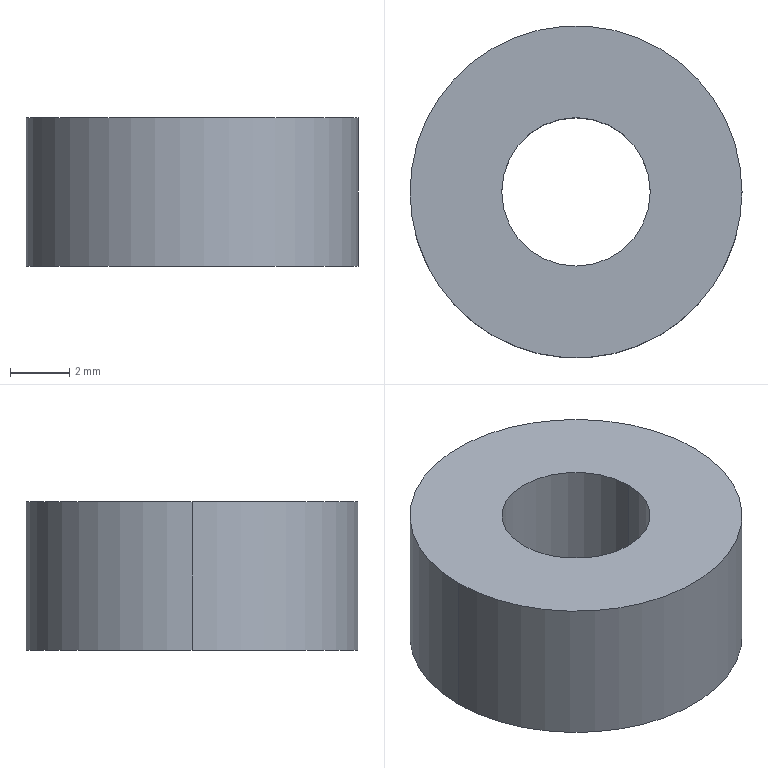Part | SolidWorks | features Extrusion 1 | 1 solid | 6 faces | box 11.179 x 11.179 x 5 mm | volume 392.607 mm3 | cylinder 4 | plane 2 | commonest cylinder face diameters 5 x2 11.179 x2
STEP:
#1=CARTESIAN_POINT('',(-2.5,0.,5.));
#2=VERTEX_POINT('',#1);
#3=CARTESIAN_POINT('',(2.5,0.,5.));
#4=VERTEX_POINT('',#3);
#5=CARTESIAN_POINT('',(0.,0.,5.));
#6=DIRECTION('',(0.,0.,1.));
#7=DIRECTION('',(1.,0.,0.));
#8=AXIS2_PLACEMENT_3D('',#5,#6,#7);
#9=CIRCLE('',#8,2.5);
#10=EDGE_CURVE('',#2,#4,#9,.T.);
#11=ORIENTED_EDGE('',*,*,#10,.T.);
#12=CARTESIAN_POINT('',(2.5,0.,0.));
#13=VERTEX_POINT('',#12);
#14=CARTESIAN_POINT('',(2.5,0.,5.));
#15=DIRECTION('',(0.,0.,-1.));
#16=VECTOR('',#15,1000.);
#17=LINE('',#14,#16);
#18=EDGE_CURVE('',#4,#13,#17,.T.);
#19=ORIENTED_EDGE('',*,*,#18,.T.);
#20=CARTESIAN_POINT('',(-2.5,0.,0.));
#21=VERTEX_POINT('',#20);
#22=CARTESIAN_POINT('',(0.,0.,0.));
#23=DIRECTION('',(0.,0.,1.));
#24=DIRECTION('',(1.,0.,0.));
#25=AXIS2_PLACEMENT_3D('',#22,#23,#24);
#26=CIRCLE('',#25,2.5);
#27=EDGE_CURVE('',#21,#13,#26,.T.);
#28=ORIENTED_EDGE('',*,*,#27,.F.);
#29=CARTESIAN_POINT('',(-2.5,0.,5.));
#30=DIRECTION('',(0.,0.,-1.));
#31=VECTOR('',#30,1000.);
#32=LINE('',#29,#31);
#33=EDGE_CURVE('',#2,#21,#32,.T.);
#34=ORIENTED_EDGE('',*,*,#33,.F.);
#35=EDGE_LOOP('',(#11,#19,#28,#34));
#36=FACE_OUTER_BOUND('',#35,.T.);
#37=CARTESIAN_POINT('',(0.,0.,5.));
#38=DIRECTION('',(0.,0.,-1.));
#39=DIRECTION('',(-1.,0.,0.));
#40=AXIS2_PLACEMENT_3D('',#37,#38,#39);
#41=CYLINDRICAL_SURFACE('',#40,2.5);
#42=ADVANCED_FACE('',(#36),#41,.F.);
#43=CARTESIAN_POINT('',(5.59,0.,5.));
#44=VERTEX_POINT('',#43);
#45=CARTESIAN_POINT('',(-5.59,0.,5.));
#46=VERTEX_POINT('',#45);
#47=CARTESIAN_POINT('',(0.,0.,5.));
#48=DIRECTION('',(0.,0.,1.));
#49=DIRECTION('',(1.,0.,0.));
#50=AXIS2_PLACEMENT_3D('',#47,#48,#49);
#51=CIRCLE('',#50,5.59);
#52=EDGE_CURVE('',#44,#46,#51,.T.);
#53=ORIENTED_EDGE('',*,*,#52,.F.);
#54=CARTESIAN_POINT('',(5.59,0.,0.));
#55=VERTEX_POINT('',#54);
#56=CARTESIAN_POINT('',(5.59,0.,5.));
#57=DIRECTION('',(0.,0.,-1.));
#58=VECTOR('',#57,1000.);
#59=LINE('',#56,#58);
#60=EDGE_CURVE('',#44,#55,#59,.T.);
#61=ORIENTED_EDGE('',*,*,#60,.T.);
#62=CARTESIAN_POINT('',(-5.59,0.,0.));
#63=VERTEX_POINT('',#62);
#64=CARTESIAN_POINT('',(0.,0.,0.));
#65=DIRECTION('',(0.,0.,1.));
#66=DIRECTION('',(1.,0.,0.));
#67=AXIS2_PLACEMENT_3D('',#64,#65,#66);
#68=CIRCLE('',#67,5.59);
#69=EDGE_CURVE('',#55,#63,#68,.T.);
#70=ORIENTED_EDGE('',*,*,#69,.T.);
#71=CARTESIAN_POINT('',(-5.59,0.,5.));
#72=DIRECTION('',(0.,0.,-1.));
#73=VECTOR('',#72,1000.);
#74=LINE('',#71,#73);
#75=EDGE_CURVE('',#46,#63,#74,.T.);
#76=ORIENTED_EDGE('',*,*,#75,.F.);
#77=EDGE_LOOP('',(#53,#61,#70,#76));
#78=FACE_OUTER_BOUND('',#77,.T.);
#79=CARTESIAN_POINT('',(0.,0.,5.));
#80=DIRECTION('',(0.,0.,-1.));
#81=DIRECTION('',(-1.,0.,0.));
#82=AXIS2_PLACEMENT_3D('',#79,#80,#81);
#83=CYLINDRICAL_SURFACE('',#82,5.59);
#84=ADVANCED_FACE('',(#78),#83,.T.);
#85=CARTESIAN_POINT('',(0.,0.,5.));
#86=DIRECTION('',(0.,0.,1.));
#87=DIRECTION('',(1.,0.,0.));
#88=AXIS2_PLACEMENT_3D('',#85,#86,#87);
#89=CIRCLE('',#88,5.59);
#90=EDGE_CURVE('',#46,#44,#89,.T.);
#91=ORIENTED_EDGE('',*,*,#90,.T.);
#92=ORIENTED_EDGE('',*,*,#52,.T.);
#93=EDGE_LOOP('',(#91,#92));
#94=FACE_OUTER_BOUND('',#93,.T.);
#95=ORIENTED_EDGE('',*,*,#10,.F.);
#96=CARTESIAN_POINT('',(0.,0.,5.));
#97=DIRECTION('',(0.,0.,1.));
#98=DIRECTION('',(1.,0.,0.));
#99=AXIS2_PLACEMENT_3D('',#96,#97,#98);
#100=CIRCLE('',#99,2.5);
#101=EDGE_CURVE('',#4,#2,#100,.T.);
#102=ORIENTED_EDGE('',*,*,#101,.F.);
#103=EDGE_LOOP('',(#95,#102));
#104=FACE_BOUND('',#103,.T.);
#105=CARTESIAN_POINT('',(0.,0.,5.));
#106=DIRECTION('',(0.,0.,1.));
#107=DIRECTION('',(1.,0.,0.));
#108=AXIS2_PLACEMENT_3D('',#105,#106,#107);
#109=PLANE('',#108);
#110=ADVANCED_FACE('',(#94,#104),#109,.T.);
#111=CARTESIAN_POINT('',(0.,0.,0.));
#112=DIRECTION('',(0.,0.,1.));
#113=DIRECTION('',(1.,0.,0.));
#114=AXIS2_PLACEMENT_3D('',#111,#112,#113);
#115=CIRCLE('',#114,5.59);
#116=EDGE_CURVE('',#63,#55,#115,.T.);
#117=ORIENTED_EDGE('',*,*,#116,.F.);
#118=ORIENTED_EDGE('',*,*,#69,.F.);
#119=EDGE_LOOP('',(#117,#118));
#120=FACE_OUTER_BOUND('',#119,.T.);
#121=ORIENTED_EDGE('',*,*,#27,.T.);
#122=CARTESIAN_POINT('',(0.,0.,0.));
#123=DIRECTION('',(0.,0.,1.));
#124=DIRECTION('',(1.,0.,0.));
#125=AXIS2_PLACEMENT_3D('',#122,#123,#124);
#126=CIRCLE('',#125,2.5);
#127=EDGE_CURVE('',#13,#21,#126,.T.);
#128=ORIENTED_EDGE('',*,*,#127,.T.);
#129=EDGE_LOOP('',(#121,#128));
#130=FACE_BOUND('',#129,.T.);
#131=CARTESIAN_POINT('',(0.,0.,0.));
#132=DIRECTION('',(0.,0.,1.));
#133=DIRECTION('',(1.,0.,0.));
#134=AXIS2_PLACEMENT_3D('',#131,#132,#133);
#135=PLANE('',#134);
#136=ADVANCED_FACE('',(#120,#130),#135,.F.);
#137=ORIENTED_EDGE('',*,*,#60,.F.);
#138=ORIENTED_EDGE('',*,*,#90,.F.);
#139=ORIENTED_EDGE('',*,*,#75,.T.);
#140=ORIENTED_EDGE('',*,*,#116,.T.);
#141=EDGE_LOOP('',(#137,#138,#139,#140));
#142=FACE_OUTER_BOUND('',#141,.T.);
#143=CARTESIAN_POINT('',(0.,0.,5.));
#144=DIRECTION('',(0.,0.,-1.));
#145=DIRECTION('',(-1.,0.,0.));
#146=AXIS2_PLACEMENT_3D('',#143,#144,#145);
#147=CYLINDRICAL_SURFACE('',#146,5.59);
#148=ADVANCED_FACE('',(#142),#147,.T.);
#149=ORIENTED_EDGE('',*,*,#18,.F.);
#150=ORIENTED_EDGE('',*,*,#101,.T.);
#151=ORIENTED_EDGE('',*,*,#33,.T.);
#152=ORIENTED_EDGE('',*,*,#127,.F.);
#153=EDGE_LOOP('',(#149,#150,#151,#152));
#154=FACE_OUTER_BOUND('',#153,.T.);
#155=CARTESIAN_POINT('',(0.,0.,5.));
#156=DIRECTION('',(0.,0.,-1.));
#157=DIRECTION('',(-1.,0.,0.));
#158=AXIS2_PLACEMENT_3D('',#155,#156,#157);
#159=CYLINDRICAL_SURFACE('',#158,2.5);
#160=ADVANCED_FACE('',(#154),#159,.F.);
#161=CLOSED_SHELL('',(#42,#84,#110,#136,#148,#160));
#162=MANIFOLD_SOLID_BREP('',#161);
#163=CARTESIAN_POINT('',(0.,0.,0.));
#164=DIRECTION('',(0.,0.,1.));
#165=DIRECTION('',(1.,0.,0.));
#166=AXIS2_PLACEMENT_3D('',#163,#164,#165);
#167=(LENGTH_UNIT()NAMED_UNIT(*)SI_UNIT(.MILLI.,.METRE.));
#168=UNCERTAINTY_MEASURE_WITH_UNIT(LENGTH_MEASURE(0.00001),#167,'','');
#169=(NAMED_UNIT(*)PLANE_ANGLE_UNIT()SI_UNIT($,.RADIAN.));
#170=(NAMED_UNIT(*)SI_UNIT($,.STERADIAN.)SOLID_ANGLE_UNIT());
#171=(GEOMETRIC_REPRESENTATION_CONTEXT(3)GLOBAL_UNCERTAINTY_ASSIGNED_CONTEXT((#168))GLOBAL_UNIT_ASSIGNED_CONTEXT((#167,#169,#170))REPRESENTATION_CONTEXT('',''));
#172=ADVANCED_BREP_SHAPE_REPRESENTATION('',(#162,#166),#171);